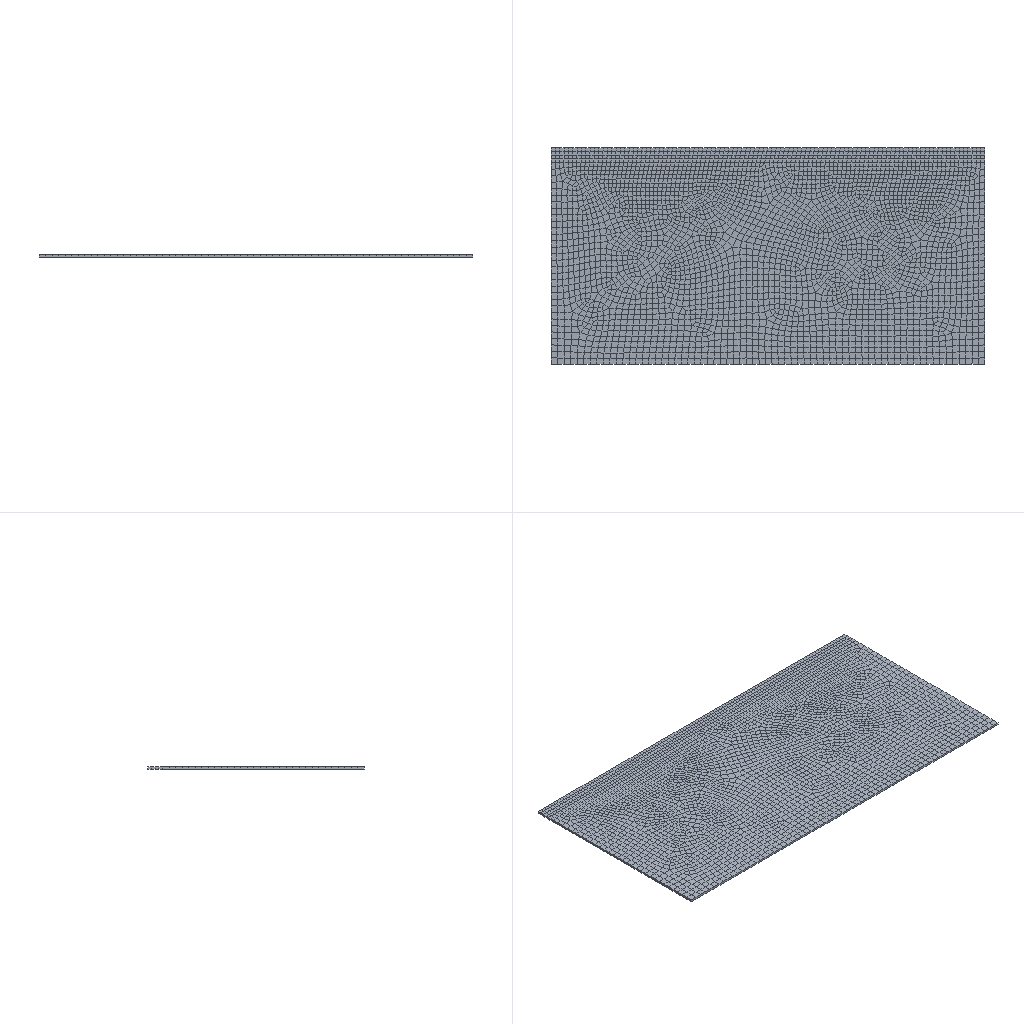Simulation study | abaqus
Set-up summary:
category,name,step,type,value,unit,region
solver,abaqus
solver,version,,,Abaqus/Standard 2020
units,not stated in the deck,,not stated
analysis,deck,,static,static
load_step,Step-1,Step-1,static
load_step,requested,,,1
mesh,nodes,,,7742
mesh,elements,,,3733
element_type,C3D8R,,solid,3733
load,load commands in deck,,count,1
bc,support commands in deck,,count,1
material,TC4,,in results
material,TIN,,in results
check,setup vs results,,match,"per instance, exact: element labels, types and connectivity; labels of the nodes the elements use; coordinates of those nodes at SINGLE_PRECISION in 1 of 1 instance(s)"
Abaqus input file, long lists of numbers shortened:
*Heading
** Job name: Job-1 Model name: Model-1
** Generated by: Abaqus/CAE 2020
*Preprint, echo=NO, model=NO, history=NO, contact=NO
**
** PARTS
**
*Part, name=Part-3
*End Part
**
**
** ASSEMBLY
**
*Assembly, name=Assembly
**
*Instance, name=Part-3-1, part=Part-3
   -5.064,     2.915,           0.
*Node
      1,   5.064,  -2.915, 0.001
      2,   5.062,  -2.922, 0.001
** (7740 more lines like these left out)
*Element, type=C3D8R
  1,    8,  131,  897,  185,    1,   23,  747,  128
  2,  131,  130,  898,  897,   23,   24,  748,  747
** (3731 more lines like these left out)
*Nset, nset=Set-3
    1,    2,    3,    4,    5,    6,    7,    8,    9,   10,   11,   12,   23,   24,   25,   26
   27,   28,   29,   30,   31,   32,   33,   34,   35,   36,   37,   38,   39,   40,   41,   42
** (63 more lines like these left out)
*Elset, elset=Set-3, generate
   1,  404,    1
*Nset, nset=Set-4
    2,    3,    5,    6,    9,   10,   13,   14,   15,   16,   17,   18,   19,   20,   21,   22
   26,   27,   28,   29,   30,   31,   32,   33,   34,   35,   36,   37,   38,   39,   40,   41
** (431 more lines like these left out)
*Elset, elset=Set-4, generate
  405,  3733,     1
** Section: TiN
*Solid Section, elset=Set-3, material=TiN
,
** Section: TC4
*Solid Section, elset=Set-4, material=TC4
,
*End Instance
**
*Nset, nset=Set-4, instance=Part-3-1
  13,  16,  18,  19, 497, 498, 499, 500, 501, 502, 503, 504, 505, 506, 507, 508
 509, 510, 511, 512, 513, 514, 515, 516, 517, 518, 519, 520, 521, 522, 523, 524
** (2 more lines like these left out)
*Elset, elset=Set-4, instance=Part-3-1
 405, 414, 478, 479, 507, 512, 517, 520, 522, 523, 524, 525, 526, 527, 528, 529
 530, 531, 532, 583, 587, 612, 614, 622, 669, 672, 676, 685, 718, 720
*Nset, nset=Set-5, instance=Part-3-1
    1,    2,    5,    8,   14,   15,   17,   20,   23,   24,   25,  129,  130,  131,  455,  456
  457,  458,  459,  460,  461,  462,  463,  464,  465,  466,  603,  604,  605,  606,  607,  608
** (3 more lines like these left out)
*Elset, elset=Set-5, instance=Part-3-1
    1,    2,    3,    4,  401,  402,  403,  404,  410,  426,  427,  436,  544,  545,  549,  553
  555,  562,  570,  575,  578, 2051, 2052, 2108, 2172, 2180, 2220, 2222, 2331, 2433, 2638, 2639
** (1 more lines like these left out)
*Nset, nset=Set-6, instance=Part-3-1
    1,    2,    5,    8,   14,   15,   17,   20,   23,   24,   25,  129,  130,  131,  455,  456
  457,  458,  459,  460,  461,  462,  463,  464,  465,  466,  603,  604,  605,  606,  607,  608
** (3 more lines like these left out)
*Elset, elset=Set-6, instance=Part-3-1
    1,    2,    3,    4,  401,  402,  403,  404,  410,  426,  427,  436,  544,  545,  549,  553
  555,  562,  570,  575,  578, 2051, 2052, 2108, 2172, 2180, 2220, 2222, 2331, 2433, 2638, 2639
** (1 more lines like these left out)
*Nset, nset=Set-8, instance=Part-3-1
  13,  16,  18,  19,  21,  22, 497, 498, 499, 500, 501, 502, 503, 504, 505, 506
 507, 508, 509, 510, 511, 512, 513, 514, 515, 516, 517, 518, 519, 520, 521, 522
** (7 more lines like these left out)
*Elset, elset=Set-8, instance=Part-3-1
  405,  414,  478,  479,  507,  512,  517,  520,  522,  523,  524,  525,  526,  527,  528,  529
  530,  531,  532,  583,  587,  612,  614,  622,  669,  672,  676,  685,  718,  720, 1977, 1987
** (3 more lines like these left out)
*Nset, nset=_PickedSet21, internal, instance=Part-3-1
    2,    3,    5,    6,    9,   10,   13,   14,   15,   16,   17,   18,   19,   20,   21,   22
   26,   27,   28,   29,   30,   31,   32,   33,   34,   35,   36,   37,   38,   39,   40,   41
** (431 more lines like these left out)
*Elset, elset=_PickedSet21, internal, instance=Part-3-1, generate
  405,  3733,     1
*Nset, nset=_PickedSet22, internal, instance=Part-3-1
 14, 17
*Elset, elset=_PickedSet22, internal, instance=Part-3-1
  410, 2743
*Elset, elset=_Surf-2_S5, internal, instance=Part-3-1, generate
 208,  404,    4
*Surface, type=ELEMENT, name=Surf-2
_Surf-2_S5, S5
*Elset, elset=_Surf-3_S5, internal, instance=Part-3-1, generate
 208,  404,    4
*Elset, elset=_Surf-3_S6, internal, instance=Part-3-1, generate
   1,  201,    4
*Surface, type=ELEMENT, name=Surf-3
_Surf-3_S5, S5
_Surf-3_S6, S6
*Nset, nset=_PickedSet21-1_, internal, instance=Part-3-1
    2,    3,   10,   13,   14,   15,   16,   21,   26,   27,   28,   29,   30,   31,   32,   33
   34,   35,   36,   37,   38,   39,   40,   41,   42,   43,   44,   45,   46,   47,   48,   49
** (215 more lines like these left out)
*Nset, nset=_PickedSet22-1_, internal, instance=Part-3-1
 14,
*Nset, nset=_PickedSet21-2_, internal, instance=Part-3-1
    5,    6,    9,   17,   18,   19,   20,   22,  132,  133,  134,  135,  136,  137,  138,  139
  140,  141,  142,  143,  144,  145,  146,  147,  148,  149,  150,  151,  152,  153,  154,  155
** (215 more lines like these left out)
*Nset, nset=_PickedSet22-2_, internal, instance=Part-3-1
 17,
*End Assembly
*Amplitude, name=Amp-1, definition=PERIODIC
1,           25.12,              0.,              0.
            2.5,              0.
**
** MATERIALS
**
*Material, name=TC4
*Elastic
112000., 0.35
*Material, name=TiN
*Elastic
400000., 0.25
**
** INTERACTION PROPERTIES
**
*Surface Interaction, name=IntProp-1
1.,
*Surface Behavior, pressure-overclosure=HARD
** ----------------------------------------------------------------
**
** STEP: Step-1
**
*Step, name=Step-1, nlgeom=YES, inc=10000
*Static, stabilize=0.0002, allsdtol=0.05, continue=NO
0.01, 1., 1e-05, 1.
**
** BOUNDARY CONDITIONS
**
** Name: BC-1 Type: 对称/反对称/完全固定
*Boundary
Set-8, ENCASTRE
**
** LOADS
**
** Name: Load-1   Type: Pressure
*Dsload, amplitude=Amp-1
Surf-3, P, 1.
**
** OUTPUT REQUESTS
**
*Restart, write, frequency=0
**
** FIELD OUTPUT: F-Output-2
**
*Output, field
*Node Output
PHILSM, PSILSM
*Element Output, directions=YES
CFAILURE, DAMAGEC, DAMAGET, ENRRTXFEM, JK, SDEG
*Contact Output
BDSTAT, CRSTS, CSDMG, DBS, DBSF, DBT, EFENRRTR, ENRRT, OPENBC
**
** FIELD OUTPUT: F-Output-1
**
*Node Output
CF, PHILSM, PSILSM, RF, U
*Element Output, directions=YES
E, ENRRTXFEM, LE, LOADSXFEM, MISES, PE, PEEQ, PEMAG, S, SDEG, STATUSXFEM
*Contact Output
CDISP, CSTRESS
*Output, history, frequency=0
**
** HISTORY OUTPUT: H-Output-1
**
*Contour Integral, crack name=H-Output-1_Crack-1, contours=4, crack tip nodes, type=K FACTORS
_PickedSet21-1_, _PickedSet22-1_, 0.53, 0.848, 0.
_PickedSet21-2_, _PickedSet22-2_, 0.53, 0.848, 0.
*End Step
Results summary:
result,step,,completed,increments=25 time=1.0/1.0
result,analysis,,,static
result,last_loadstep,,,1
result,primary field,,,U
result,reaction total,,FX,0.0,model units
result,reaction total,,FY,0.0005,model units
result,reaction total,,FZ,-0.0,model units